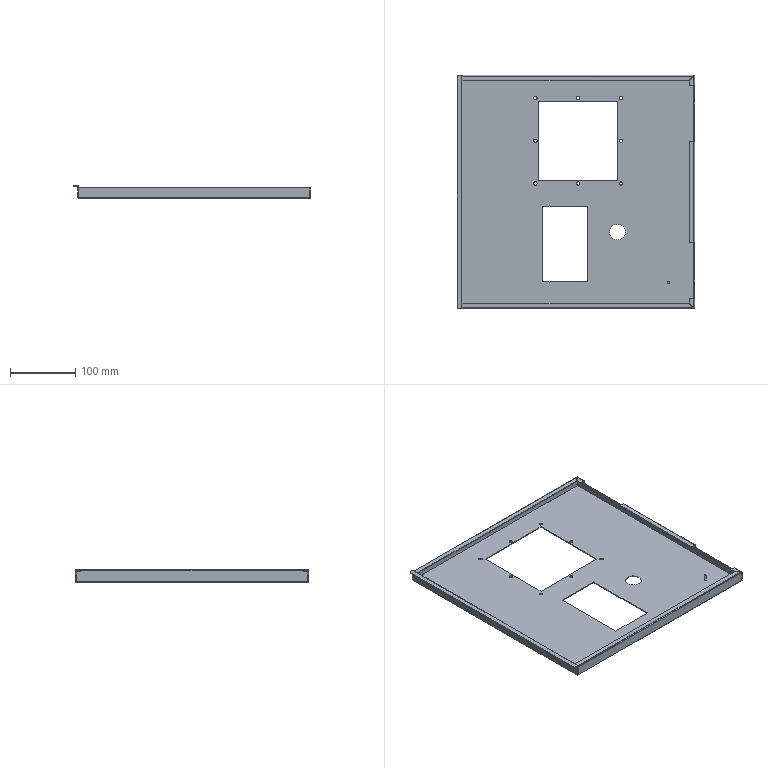Part | STEP file | Left door panel | 1 solid | 129 faces | box 362.8 x 357 x 19 mm | volume 160795 mm3 | plane 83 | cylinder 42 | spline 4 | commonest cylinder face diameters 5 x16 0.02 x10 2.42 x10 3 x2 4 x2 24 x2